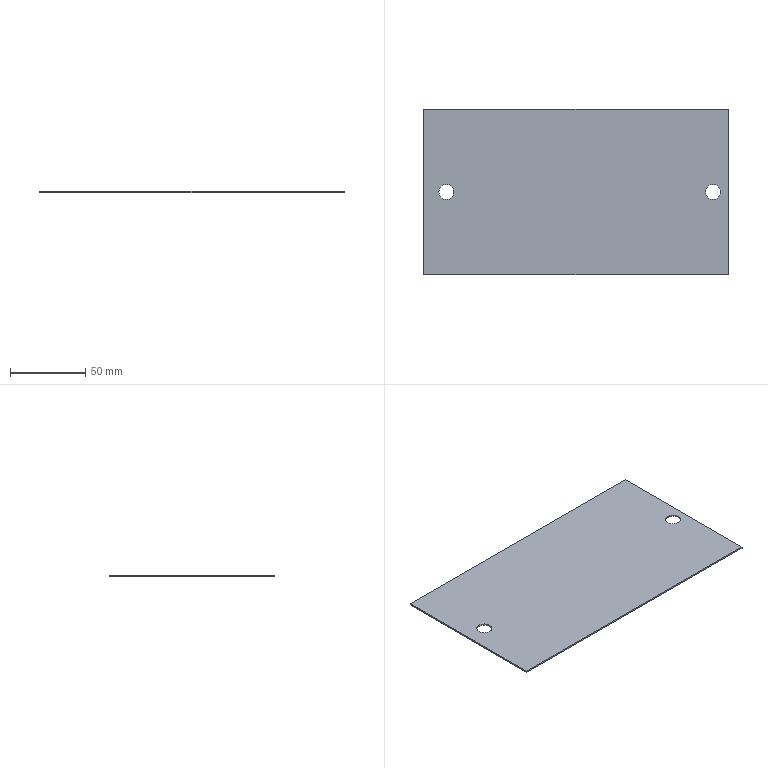Part | STEP file | 1 solid | 10 faces | box 202.5 x 110 x 1 mm | volume 22118 mm3 | plane 6 | cylinder 4 | commonest cylinder face diameters 10 x4
STEP:
#1=CARTESIAN_POINT('',(0.,0.,0.));
#2=DIRECTION('',(0.,0.,1.));
#3=DIRECTION('',(1.,0.,0.));
#4=AXIS2_PLACEMENT_3D('',#1,#2,#3);
#5=CARTESIAN_POINT('',(134.208,-8.441,1.));
#6=VERTEX_POINT('',#5);
#7=CARTESIAN_POINT('',(134.208,-8.441,0.));
#8=VERTEX_POINT('',#7);
#9=CARTESIAN_POINT('',(134.208,-8.441,1.));
#10=DIRECTION('',(0.,0.,-1.));
#11=VECTOR('',#10,1.);
#12=LINE('',#9,#11);
#13=CARTESIAN_POINT('',(139.208,-8.441,1.));
#14=DIRECTION('',(0.,0.,-1.));
#15=DIRECTION('',(-1.,0.,0.));
#16=AXIS2_PLACEMENT_3D('',#13,#14,#15);
#17=CYLINDRICAL_SURFACE('',#16,5.);
#18=CARTESIAN_POINT('',(6.283,0.));
#19=DIRECTION('',(0.,1.));
#20=VECTOR('',#19,1.);
#21=LINE('',#18,#20);
#22=(GEOMETRIC_REPRESENTATION_CONTEXT(2)PARAMETRIC_REPRESENTATION_CONTEXT()REPRESENTATION_CONTEXT('',''));
#23=DEFINITIONAL_REPRESENTATION('',(#21),#22);
#24=PCURVE('',#17,#23);
#25=CARTESIAN_POINT('',(139.208,-8.441,1.));
#26=DIRECTION('',(0.,0.,-1.));
#27=DIRECTION('',(-1.,0.,0.));
#28=AXIS2_PLACEMENT_3D('',#25,#26,#27);
#29=CYLINDRICAL_SURFACE('',#28,5.);
#30=CARTESIAN_POINT('',(0.,0.));
#31=DIRECTION('',(0.,1.));
#32=VECTOR('',#31,1.);
#33=LINE('',#30,#32);
#34=(GEOMETRIC_REPRESENTATION_CONTEXT(2)PARAMETRIC_REPRESENTATION_CONTEXT()REPRESENTATION_CONTEXT('',''));
#35=DEFINITIONAL_REPRESENTATION('',(#33),#34);
#36=PCURVE('',#29,#35);
#37=SURFACE_CURVE('',#12,(#24,#36),.PCURVE_S1.);
#38=EDGE_CURVE('',#6,#8,#37,.T.);
#39=ORIENTED_EDGE('',*,*,#38,.T.);
#40=CARTESIAN_POINT('',(144.208,-8.441,0.));
#41=VERTEX_POINT('',#40);
#42=CARTESIAN_POINT('',(139.208,-8.441,0.));
#43=DIRECTION('',(0.,0.,-1.));
#44=DIRECTION('',(-1.,0.,0.));
#45=AXIS2_PLACEMENT_3D('',#42,#43,#44);
#46=CIRCLE('',#45,5.);
#47=CARTESIAN_POINT('',(0.,1.));
#48=DIRECTION('',(1.,0.));
#49=VECTOR('',#48,1.);
#50=LINE('',#47,#49);
#51=(GEOMETRIC_REPRESENTATION_CONTEXT(2)PARAMETRIC_REPRESENTATION_CONTEXT()REPRESENTATION_CONTEXT('',''));
#52=DEFINITIONAL_REPRESENTATION('',(#50),#51);
#53=PCURVE('',#17,#52);
#54=CARTESIAN_POINT('',(47.958,-8.441,0.));
#55=DIRECTION('',(0.,0.,1.));
#56=DIRECTION('',(1.,0.,0.));
#57=AXIS2_PLACEMENT_3D('',#54,#55,#56);
#58=PLANE('',#57);
#59=CARTESIAN_POINT('',(86.25,0.));
#60=CARTESIAN_POINT('',(86.25,8.66));
#61=CARTESIAN_POINT('',(93.75,4.33));
#62=CARTESIAN_POINT('',(101.25,0.));
#63=CARTESIAN_POINT('',(93.75,-4.33));
#64=CARTESIAN_POINT('',(86.25,-8.66));
#65=CARTESIAN_POINT('',(86.25,0.));
#66=(BOUNDED_CURVE()B_SPLINE_CURVE(2,(#59,#60,#61,#62,#63,#64,#65),.UNSPECIFIED.,.T.,.F.)B_SPLINE_CURVE_WITH_KNOTS((1,2,2,2,2,1),(-2.094,0.,2.094,4.189,6.283,8.378),.UNSPECIFIED.)CURVE()GEOMETRIC_REPRESENTATION_ITEM()RATIONAL_B_SPLINE_CURVE((1.,0.5,1.,0.5,1.,0.5,1.))REPRESENTATION_ITEM(''));
#67=(GEOMETRIC_REPRESENTATION_CONTEXT(2)PARAMETRIC_REPRESENTATION_CONTEXT()REPRESENTATION_CONTEXT('',''));
#68=DEFINITIONAL_REPRESENTATION('',(#66),#67);
#69=PCURVE('',#58,#68);
#70=SURFACE_CURVE('',#46,(#53,#69),.PCURVE_S1.);
#71=EDGE_CURVE('',#41,#8,#70,.T.);
#72=ORIENTED_EDGE('',*,*,#71,.F.);
#73=CARTESIAN_POINT('',(144.208,-8.441,1.));
#74=VERTEX_POINT('',#73);
#75=CARTESIAN_POINT('',(144.208,-8.441,1.));
#76=DIRECTION('',(0.,0.,-1.));
#77=VECTOR('',#76,1.);
#78=LINE('',#75,#77);
#79=CARTESIAN_POINT('',(3.142,0.));
#80=DIRECTION('',(0.,1.));
#81=VECTOR('',#80,1.);
#82=LINE('',#79,#81);
#83=(GEOMETRIC_REPRESENTATION_CONTEXT(2)PARAMETRIC_REPRESENTATION_CONTEXT()REPRESENTATION_CONTEXT('',''));
#84=DEFINITIONAL_REPRESENTATION('',(#82),#83);
#85=PCURVE('',#17,#84);
#86=CARTESIAN_POINT('',(3.142,0.));
#87=DIRECTION('',(0.,1.));
#88=VECTOR('',#87,1.);
#89=LINE('',#86,#88);
#90=(GEOMETRIC_REPRESENTATION_CONTEXT(2)PARAMETRIC_REPRESENTATION_CONTEXT()REPRESENTATION_CONTEXT('',''));
#91=DEFINITIONAL_REPRESENTATION('',(#89),#90);
#92=PCURVE('',#29,#91);
#93=SURFACE_CURVE('',#78,(#85,#92),.PCURVE_S1.);
#94=EDGE_CURVE('',#74,#41,#93,.T.);
#95=ORIENTED_EDGE('',*,*,#94,.F.);
#96=CARTESIAN_POINT('',(139.208,-8.441,1.));
#97=DIRECTION('',(0.,0.,-1.));
#98=DIRECTION('',(-1.,0.,0.));
#99=AXIS2_PLACEMENT_3D('',#96,#97,#98);
#100=CIRCLE('',#99,5.);
#101=CARTESIAN_POINT('',(0.,0.));
#102=DIRECTION('',(1.,0.));
#103=VECTOR('',#102,1.);
#104=LINE('',#101,#103);
#105=(GEOMETRIC_REPRESENTATION_CONTEXT(2)PARAMETRIC_REPRESENTATION_CONTEXT()REPRESENTATION_CONTEXT('',''));
#106=DEFINITIONAL_REPRESENTATION('',(#104),#105);
#107=PCURVE('',#17,#106);
#108=CARTESIAN_POINT('',(47.958,-8.441,1.));
#109=DIRECTION('',(0.,0.,1.));
#110=DIRECTION('',(1.,0.,0.));
#111=AXIS2_PLACEMENT_3D('',#108,#109,#110);
#112=PLANE('',#111);
#113=CARTESIAN_POINT('',(86.25,0.));
#114=CARTESIAN_POINT('',(86.25,8.66));
#115=CARTESIAN_POINT('',(93.75,4.33));
#116=CARTESIAN_POINT('',(101.25,0.));
#117=CARTESIAN_POINT('',(93.75,-4.33));
#118=CARTESIAN_POINT('',(86.25,-8.66));
#119=CARTESIAN_POINT('',(86.25,0.));
#120=(BOUNDED_CURVE()B_SPLINE_CURVE(2,(#113,#114,#115,#116,#117,#118,#119),.UNSPECIFIED.,.T.,.F.)B_SPLINE_CURVE_WITH_KNOTS((1,2,2,2,2,1),(-2.094,0.,2.094,4.189,6.283,8.378),.UNSPECIFIED.)CURVE()GEOMETRIC_REPRESENTATION_ITEM()RATIONAL_B_SPLINE_CURVE((1.,0.5,1.,0.5,1.,0.5,1.))REPRESENTATION_ITEM(''));
#121=(GEOMETRIC_REPRESENTATION_CONTEXT(2)PARAMETRIC_REPRESENTATION_CONTEXT()REPRESENTATION_CONTEXT('',''));
#122=DEFINITIONAL_REPRESENTATION('',(#120),#121);
#123=PCURVE('',#112,#122);
#124=SURFACE_CURVE('',#100,(#107,#123),.PCURVE_S1.);
#125=EDGE_CURVE('',#74,#6,#124,.T.);
#126=ORIENTED_EDGE('',*,*,#125,.T.);
#127=EDGE_LOOP('',(#39,#72,#95,#126));
#128=FACE_BOUND('',#127,.F.);
#129=ADVANCED_FACE('',(#128),#17,.F.);
#130=CARTESIAN_POINT('',(-43.292,-8.441,1.));
#131=VERTEX_POINT('',#130);
#132=CARTESIAN_POINT('',(-43.292,-8.441,0.));
#133=VERTEX_POINT('',#132);
#134=CARTESIAN_POINT('',(-43.292,-8.441,1.));
#135=DIRECTION('',(0.,0.,-1.));
#136=VECTOR('',#135,1.);
#137=LINE('',#134,#136);
#138=CARTESIAN_POINT('',(-38.292,-8.441,1.));
#139=DIRECTION('',(0.,0.,-1.));
#140=DIRECTION('',(-1.,0.,0.));
#141=AXIS2_PLACEMENT_3D('',#138,#139,#140);
#142=CYLINDRICAL_SURFACE('',#141,5.);
#143=CARTESIAN_POINT('',(6.283,0.));
#144=DIRECTION('',(0.,1.));
#145=VECTOR('',#144,1.);
#146=LINE('',#143,#145);
#147=(GEOMETRIC_REPRESENTATION_CONTEXT(2)PARAMETRIC_REPRESENTATION_CONTEXT()REPRESENTATION_CONTEXT('',''));
#148=DEFINITIONAL_REPRESENTATION('',(#146),#147);
#149=PCURVE('',#142,#148);
#150=CARTESIAN_POINT('',(-38.292,-8.441,1.));
#151=DIRECTION('',(0.,0.,-1.));
#152=DIRECTION('',(-1.,0.,0.));
#153=AXIS2_PLACEMENT_3D('',#150,#151,#152);
#154=CYLINDRICAL_SURFACE('',#153,5.);
#155=CARTESIAN_POINT('',(0.,0.));
#156=DIRECTION('',(0.,1.));
#157=VECTOR('',#156,1.);
#158=LINE('',#155,#157);
#159=(GEOMETRIC_REPRESENTATION_CONTEXT(2)PARAMETRIC_REPRESENTATION_CONTEXT()REPRESENTATION_CONTEXT('',''));
#160=DEFINITIONAL_REPRESENTATION('',(#158),#159);
#161=PCURVE('',#154,#160);
#162=SURFACE_CURVE('',#137,(#149,#161),.PCURVE_S1.);
#163=EDGE_CURVE('',#131,#133,#162,.T.);
#164=ORIENTED_EDGE('',*,*,#163,.T.);
#165=CARTESIAN_POINT('',(-33.292,-8.441,0.));
#166=VERTEX_POINT('',#165);
#167=CARTESIAN_POINT('',(-38.292,-8.441,0.));
#168=DIRECTION('',(0.,0.,-1.));
#169=DIRECTION('',(-1.,0.,0.));
#170=AXIS2_PLACEMENT_3D('',#167,#168,#169);
#171=CIRCLE('',#170,5.);
#172=CARTESIAN_POINT('',(0.,1.));
#173=DIRECTION('',(1.,0.));
#174=VECTOR('',#173,1.);
#175=LINE('',#172,#174);
#176=(GEOMETRIC_REPRESENTATION_CONTEXT(2)PARAMETRIC_REPRESENTATION_CONTEXT()REPRESENTATION_CONTEXT('',''));
#177=DEFINITIONAL_REPRESENTATION('',(#175),#176);
#178=PCURVE('',#142,#177);
#179=CARTESIAN_POINT('',(-91.25,0.));
#180=CARTESIAN_POINT('',(-91.25,8.66));
#181=CARTESIAN_POINT('',(-83.75,4.33));
#182=CARTESIAN_POINT('',(-76.25,0.));
#183=CARTESIAN_POINT('',(-83.75,-4.33));
#184=CARTESIAN_POINT('',(-91.25,-8.66));
#185=CARTESIAN_POINT('',(-91.25,0.));
#186=(BOUNDED_CURVE()B_SPLINE_CURVE(2,(#179,#180,#181,#182,#183,#184,#185),.UNSPECIFIED.,.T.,.F.)B_SPLINE_CURVE_WITH_KNOTS((1,2,2,2,2,1),(-2.094,0.,2.094,4.189,6.283,8.378),.UNSPECIFIED.)CURVE()GEOMETRIC_REPRESENTATION_ITEM()RATIONAL_B_SPLINE_CURVE((1.,0.5,1.,0.5,1.,0.5,1.))REPRESENTATION_ITEM(''));
#187=(GEOMETRIC_REPRESENTATION_CONTEXT(2)PARAMETRIC_REPRESENTATION_CONTEXT()REPRESENTATION_CONTEXT('',''));
#188=DEFINITIONAL_REPRESENTATION('',(#186),#187);
#189=PCURVE('',#58,#188);
#190=SURFACE_CURVE('',#171,(#178,#189),.PCURVE_S1.);
#191=EDGE_CURVE('',#166,#133,#190,.T.);
#192=ORIENTED_EDGE('',*,*,#191,.F.);
#193=CARTESIAN_POINT('',(-33.292,-8.441,1.));
#194=VERTEX_POINT('',#193);
#195=CARTESIAN_POINT('',(-33.292,-8.441,1.));
#196=DIRECTION('',(0.,0.,-1.));
#197=VECTOR('',#196,1.);
#198=LINE('',#195,#197);
#199=CARTESIAN_POINT('',(3.142,0.));
#200=DIRECTION('',(0.,1.));
#201=VECTOR('',#200,1.);
#202=LINE('',#199,#201);
#203=(GEOMETRIC_REPRESENTATION_CONTEXT(2)PARAMETRIC_REPRESENTATION_CONTEXT()REPRESENTATION_CONTEXT('',''));
#204=DEFINITIONAL_REPRESENTATION('',(#202),#203);
#205=PCURVE('',#142,#204);
#206=CARTESIAN_POINT('',(3.142,0.));
#207=DIRECTION('',(0.,1.));
#208=VECTOR('',#207,1.);
#209=LINE('',#206,#208);
#210=(GEOMETRIC_REPRESENTATION_CONTEXT(2)PARAMETRIC_REPRESENTATION_CONTEXT()REPRESENTATION_CONTEXT('',''));
#211=DEFINITIONAL_REPRESENTATION('',(#209),#210);
#212=PCURVE('',#154,#211);
#213=SURFACE_CURVE('',#198,(#205,#212),.PCURVE_S1.);
#214=EDGE_CURVE('',#194,#166,#213,.T.);
#215=ORIENTED_EDGE('',*,*,#214,.F.);
#216=CARTESIAN_POINT('',(-38.292,-8.441,1.));
#217=DIRECTION('',(0.,0.,-1.));
#218=DIRECTION('',(-1.,0.,0.));
#219=AXIS2_PLACEMENT_3D('',#216,#217,#218);
#220=CIRCLE('',#219,5.);
#221=CARTESIAN_POINT('',(0.,0.));
#222=DIRECTION('',(1.,0.));
#223=VECTOR('',#222,1.);
#224=LINE('',#221,#223);
#225=(GEOMETRIC_REPRESENTATION_CONTEXT(2)PARAMETRIC_REPRESENTATION_CONTEXT()REPRESENTATION_CONTEXT('',''));
#226=DEFINITIONAL_REPRESENTATION('',(#224),#225);
#227=PCURVE('',#142,#226);
#228=CARTESIAN_POINT('',(-91.25,0.));
#229=CARTESIAN_POINT('',(-91.25,8.66));
#230=CARTESIAN_POINT('',(-83.75,4.33));
#231=CARTESIAN_POINT('',(-76.25,0.));
#232=CARTESIAN_POINT('',(-83.75,-4.33));
#233=CARTESIAN_POINT('',(-91.25,-8.66));
#234=CARTESIAN_POINT('',(-91.25,0.));
#235=(BOUNDED_CURVE()B_SPLINE_CURVE(2,(#228,#229,#230,#231,#232,#233,#234),.UNSPECIFIED.,.T.,.F.)B_SPLINE_CURVE_WITH_KNOTS((1,2,2,2,2,1),(-2.094,0.,2.094,4.189,6.283,8.378),.UNSPECIFIED.)CURVE()GEOMETRIC_REPRESENTATION_ITEM()RATIONAL_B_SPLINE_CURVE((1.,0.5,1.,0.5,1.,0.5,1.))REPRESENTATION_ITEM(''));
#236=(GEOMETRIC_REPRESENTATION_CONTEXT(2)PARAMETRIC_REPRESENTATION_CONTEXT()REPRESENTATION_CONTEXT('',''));
#237=DEFINITIONAL_REPRESENTATION('',(#235),#236);
#238=PCURVE('',#112,#237);
#239=SURFACE_CURVE('',#220,(#227,#238),.PCURVE_S1.);
#240=EDGE_CURVE('',#194,#131,#239,.T.);
#241=ORIENTED_EDGE('',*,*,#240,.T.);
#242=EDGE_LOOP('',(#164,#192,#215,#241));
#243=FACE_BOUND('',#242,.F.);
#244=ADVANCED_FACE('',(#243),#142,.F.);
#245=CARTESIAN_POINT('',(149.208,-63.441,0.));
#246=VERTEX_POINT('',#245);
#247=CARTESIAN_POINT('',(149.208,46.559,0.));
#248=VERTEX_POINT('',#247);
#249=CARTESIAN_POINT('',(149.208,-8.441,0.));
#250=DIRECTION('',(0.,1.,0.));
#251=VECTOR('',#250,1.);
#252=LINE('',#249,#251);
#253=CARTESIAN_POINT('',(101.25,0.));
#254=DIRECTION('',(0.,1.));
#255=VECTOR('',#254,1.);
#256=LINE('',#253,#255);
#257=(GEOMETRIC_REPRESENTATION_CONTEXT(2)PARAMETRIC_REPRESENTATION_CONTEXT()REPRESENTATION_CONTEXT('',''));
#258=DEFINITIONAL_REPRESENTATION('',(#256),#257);
#259=PCURVE('',#58,#258);
#260=CARTESIAN_POINT('',(149.208,-63.441,0.));
#261=DIRECTION('',(1.,0.,0.));
#262=DIRECTION('',(0.,0.,-1.));
#263=AXIS2_PLACEMENT_3D('',#260,#261,#262);
#264=PLANE('',#263);
#265=CARTESIAN_POINT('',(0.,55.));
#266=DIRECTION('',(0.,1.));
#267=VECTOR('',#266,1.);
#268=LINE('',#265,#267);
#269=(GEOMETRIC_REPRESENTATION_CONTEXT(2)PARAMETRIC_REPRESENTATION_CONTEXT()REPRESENTATION_CONTEXT('',''));
#270=DEFINITIONAL_REPRESENTATION('',(#268),#269);
#271=PCURVE('',#264,#270);
#272=SURFACE_CURVE('',#252,(#259,#271),.PCURVE_S1.);
#273=EDGE_CURVE('',#246,#248,#272,.T.);
#274=ORIENTED_EDGE('',*,*,#273,.F.);
#275=CARTESIAN_POINT('',(-53.292,-63.441,0.));
#276=VERTEX_POINT('',#275);
#277=CARTESIAN_POINT('',(47.958,-63.441,0.));
#278=DIRECTION('',(1.,0.,0.));
#279=VECTOR('',#278,1.);
#280=LINE('',#277,#279);
#281=CARTESIAN_POINT('',(0.,-55.));
#282=DIRECTION('',(1.,0.));
#283=VECTOR('',#282,1.);
#284=LINE('',#281,#283);
#285=(GEOMETRIC_REPRESENTATION_CONTEXT(2)PARAMETRIC_REPRESENTATION_CONTEXT()REPRESENTATION_CONTEXT('',''));
#286=DEFINITIONAL_REPRESENTATION('',(#284),#285);
#287=PCURVE('',#58,#286);
#288=CARTESIAN_POINT('',(-53.292,-63.441,0.));
#289=DIRECTION('',(0.,-1.,0.));
#290=DIRECTION('',(1.,0.,0.));
#291=AXIS2_PLACEMENT_3D('',#288,#289,#290);
#292=PLANE('',#291);
#293=CARTESIAN_POINT('',(101.25,0.));
#294=DIRECTION('',(1.,0.));
#295=VECTOR('',#294,1.);
#296=LINE('',#293,#295);
#297=(GEOMETRIC_REPRESENTATION_CONTEXT(2)PARAMETRIC_REPRESENTATION_CONTEXT()REPRESENTATION_CONTEXT('',''));
#298=DEFINITIONAL_REPRESENTATION('',(#296),#297);
#299=PCURVE('',#292,#298);
#300=SURFACE_CURVE('',#280,(#287,#299),.PCURVE_S1.);
#301=EDGE_CURVE('',#276,#246,#300,.T.);
#302=ORIENTED_EDGE('',*,*,#301,.F.);
#303=CARTESIAN_POINT('',(-53.292,46.559,0.));
#304=VERTEX_POINT('',#303);
#305=CARTESIAN_POINT('',(-53.292,-8.441,0.));
#306=DIRECTION('',(0.,-1.,0.));
#307=VECTOR('',#306,1.);
#308=LINE('',#305,#307);
#309=CARTESIAN_POINT('',(-101.25,0.));
#310=DIRECTION('',(0.,-1.));
#311=VECTOR('',#310,1.);
#312=LINE('',#309,#311);
#313=(GEOMETRIC_REPRESENTATION_CONTEXT(2)PARAMETRIC_REPRESENTATION_CONTEXT()REPRESENTATION_CONTEXT('',''));
#314=DEFINITIONAL_REPRESENTATION('',(#312),#313);
#315=PCURVE('',#58,#314);
#316=CARTESIAN_POINT('',(-53.292,46.559,0.));
#317=DIRECTION('',(-1.,0.,0.));
#318=DIRECTION('',(0.,-1.,0.));
#319=AXIS2_PLACEMENT_3D('',#316,#317,#318);
#320=PLANE('',#319);
#321=CARTESIAN_POINT('',(55.,0.));
#322=DIRECTION('',(1.,0.));
#323=VECTOR('',#322,1.);
#324=LINE('',#321,#323);
#325=(GEOMETRIC_REPRESENTATION_CONTEXT(2)PARAMETRIC_REPRESENTATION_CONTEXT()REPRESENTATION_CONTEXT('',''));
#326=DEFINITIONAL_REPRESENTATION('',(#324),#325);
#327=PCURVE('',#320,#326);
#328=SURFACE_CURVE('',#308,(#315,#327),.PCURVE_S1.);
#329=EDGE_CURVE('',#304,#276,#328,.T.);
#330=ORIENTED_EDGE('',*,*,#329,.F.);
#331=CARTESIAN_POINT('',(47.958,46.559,0.));
#332=DIRECTION('',(-1.,0.,0.));
#333=VECTOR('',#332,1.);
#334=LINE('',#331,#333);
#335=CARTESIAN_POINT('',(0.,55.));
#336=DIRECTION('',(-1.,0.));
#337=VECTOR('',#336,1.);
#338=LINE('',#335,#337);
#339=(GEOMETRIC_REPRESENTATION_CONTEXT(2)PARAMETRIC_REPRESENTATION_CONTEXT()REPRESENTATION_CONTEXT('',''));
#340=DEFINITIONAL_REPRESENTATION('',(#338),#339);
#341=PCURVE('',#58,#340);
#342=CARTESIAN_POINT('',(149.208,46.559,0.));
#343=DIRECTION('',(0.,1.,0.));
#344=DIRECTION('',(0.,0.,1.));
#345=AXIS2_PLACEMENT_3D('',#342,#343,#344);
#346=PLANE('',#345);
#347=CARTESIAN_POINT('',(0.,-101.25));
#348=DIRECTION('',(0.,-1.));
#349=VECTOR('',#348,1.);
#350=LINE('',#347,#349);
#351=(GEOMETRIC_REPRESENTATION_CONTEXT(2)PARAMETRIC_REPRESENTATION_CONTEXT()REPRESENTATION_CONTEXT('',''));
#352=DEFINITIONAL_REPRESENTATION('',(#350),#351);
#353=PCURVE('',#346,#352);
#354=SURFACE_CURVE('',#334,(#341,#353),.PCURVE_S1.);
#355=EDGE_CURVE('',#248,#304,#354,.T.);
#356=ORIENTED_EDGE('',*,*,#355,.F.);
#357=EDGE_LOOP('',(#274,#302,#330,#356));
#358=FACE_BOUND('',#357,.T.);
#359=CARTESIAN_POINT('',(139.208,-8.441,0.));
#360=DIRECTION('',(0.,0.,-1.));
#361=DIRECTION('',(-1.,0.,0.));
#362=AXIS2_PLACEMENT_3D('',#359,#360,#361);
#363=CIRCLE('',#362,5.);
#364=CARTESIAN_POINT('',(86.25,0.));
#365=CARTESIAN_POINT('',(86.25,8.66));
#366=CARTESIAN_POINT('',(93.75,4.33));
#367=CARTESIAN_POINT('',(101.25,0.));
#368=CARTESIAN_POINT('',(93.75,-4.33));
#369=CARTESIAN_POINT('',(86.25,-8.66));
#370=CARTESIAN_POINT('',(86.25,0.));
#371=(BOUNDED_CURVE()B_SPLINE_CURVE(2,(#364,#365,#366,#367,#368,#369,#370),.UNSPECIFIED.,.T.,.F.)B_SPLINE_CURVE_WITH_KNOTS((1,2,2,2,2,1),(-2.094,0.,2.094,4.189,6.283,8.378),.UNSPECIFIED.)CURVE()GEOMETRIC_REPRESENTATION_ITEM()RATIONAL_B_SPLINE_CURVE((1.,0.5,1.,0.5,1.,0.5,1.))REPRESENTATION_ITEM(''));
#372=(GEOMETRIC_REPRESENTATION_CONTEXT(2)PARAMETRIC_REPRESENTATION_CONTEXT()REPRESENTATION_CONTEXT('',''));
#373=DEFINITIONAL_REPRESENTATION('',(#371),#372);
#374=PCURVE('',#58,#373);
#375=CARTESIAN_POINT('',(0.,1.));
#376=DIRECTION('',(1.,0.));
#377=VECTOR('',#376,1.);
#378=LINE('',#375,#377);
#379=(GEOMETRIC_REPRESENTATION_CONTEXT(2)PARAMETRIC_REPRESENTATION_CONTEXT()REPRESENTATION_CONTEXT('',''));
#380=DEFINITIONAL_REPRESENTATION('',(#378),#379);
#381=PCURVE('',#29,#380);
#382=SURFACE_CURVE('',#363,(#374,#381),.PCURVE_S1.);
#383=EDGE_CURVE('',#8,#41,#382,.T.);
#384=ORIENTED_EDGE('',*,*,#383,.F.);
#385=ORIENTED_EDGE('',*,*,#71,.F.);
#386=EDGE_LOOP('',(#384,#385));
#387=FACE_BOUND('',#386,.T.);
#388=CARTESIAN_POINT('',(-38.292,-8.441,0.));
#389=DIRECTION('',(0.,0.,-1.));
#390=DIRECTION('',(-1.,0.,0.));
#391=AXIS2_PLACEMENT_3D('',#388,#389,#390);
#392=CIRCLE('',#391,5.);
#393=CARTESIAN_POINT('',(-91.25,0.));
#394=CARTESIAN_POINT('',(-91.25,8.66));
#395=CARTESIAN_POINT('',(-83.75,4.33));
#396=CARTESIAN_POINT('',(-76.25,0.));
#397=CARTESIAN_POINT('',(-83.75,-4.33));
#398=CARTESIAN_POINT('',(-91.25,-8.66));
#399=CARTESIAN_POINT('',(-91.25,0.));
#400=(BOUNDED_CURVE()B_SPLINE_CURVE(2,(#393,#394,#395,#396,#397,#398,#399),.UNSPECIFIED.,.T.,.F.)B_SPLINE_CURVE_WITH_KNOTS((1,2,2,2,2,1),(-2.094,0.,2.094,4.189,6.283,8.378),.UNSPECIFIED.)CURVE()GEOMETRIC_REPRESENTATION_ITEM()RATIONAL_B_SPLINE_CURVE((1.,0.5,1.,0.5,1.,0.5,1.))REPRESENTATION_ITEM(''));
#401=(GEOMETRIC_REPRESENTATION_CONTEXT(2)PARAMETRIC_REPRESENTATION_CONTEXT()REPRESENTATION_CONTEXT('',''));
#402=DEFINITIONAL_REPRESENTATION('',(#400),#401);
#403=PCURVE('',#58,#402);
#404=CARTESIAN_POINT('',(0.,1.));
#405=DIRECTION('',(1.,0.));
#406=VECTOR('',#405,1.);
#407=LINE('',#404,#406);
#408=(GEOMETRIC_REPRESENTATION_CONTEXT(2)PARAMETRIC_REPRESENTATION_CONTEXT()REPRESENTATION_CONTEXT('',''));
#409=DEFINITIONAL_REPRESENTATION('',(#407),#408);
#410=PCURVE('',#154,#409);
#411=SURFACE_CURVE('',#392,(#403,#410),.PCURVE_S1.);
#412=EDGE_CURVE('',#133,#166,#411,.T.);
#413=ORIENTED_EDGE('',*,*,#412,.F.);
#414=ORIENTED_EDGE('',*,*,#191,.F.);
#415=EDGE_LOOP('',(#413,#414));
#416=FACE_BOUND('',#415,.T.);
#417=ADVANCED_FACE('',(#358,#387,#416),#58,.F.);
#418=CARTESIAN_POINT('',(-53.292,46.559,1.));
#419=VERTEX_POINT('',#418);
#420=CARTESIAN_POINT('',(149.208,46.559,1.));
#421=VERTEX_POINT('',#420);
#422=CARTESIAN_POINT('',(149.208,46.559,1.));
#423=DIRECTION('',(1.,0.,0.));
#424=VECTOR('',#423,1.);
#425=LINE('',#422,#424);
#426=CARTESIAN_POINT('',(1.,0.));
#427=DIRECTION('',(0.,1.));
#428=VECTOR('',#427,1.);
#429=LINE('',#426,#428);
#430=(GEOMETRIC_REPRESENTATION_CONTEXT(2)PARAMETRIC_REPRESENTATION_CONTEXT()REPRESENTATION_CONTEXT('',''));
#431=DEFINITIONAL_REPRESENTATION('',(#429),#430);
#432=PCURVE('',#346,#431);
#433=CARTESIAN_POINT('',(101.25,55.));
#434=DIRECTION('',(1.,0.));
#435=VECTOR('',#434,1.);
#436=LINE('',#433,#435);
#437=(GEOMETRIC_REPRESENTATION_CONTEXT(2)PARAMETRIC_REPRESENTATION_CONTEXT()REPRESENTATION_CONTEXT('',''));
#438=DEFINITIONAL_REPRESENTATION('',(#436),#437);
#439=PCURVE('',#112,#438);
#440=SURFACE_CURVE('',#425,(#432,#439),.PCURVE_S1.);
#441=EDGE_CURVE('',#419,#421,#440,.T.);
#442=ORIENTED_EDGE('',*,*,#441,.T.);
#443=CARTESIAN_POINT('',(149.208,46.559,0.));
#444=DIRECTION('',(0.,0.,-1.));
#445=VECTOR('',#444,1.);
#446=LINE('',#443,#445);
#447=CARTESIAN_POINT('',(0.,0.));
#448=DIRECTION('',(-1.,0.));
#449=VECTOR('',#448,1.);
#450=LINE('',#447,#449);
#451=(GEOMETRIC_REPRESENTATION_CONTEXT(2)PARAMETRIC_REPRESENTATION_CONTEXT()REPRESENTATION_CONTEXT('',''));
#452=DEFINITIONAL_REPRESENTATION('',(#450),#451);
#453=PCURVE('',#346,#452);
#454=CARTESIAN_POINT('',(0.,110.));
#455=DIRECTION('',(1.,0.));
#456=VECTOR('',#455,1.);
#457=LINE('',#454,#456);
#458=(GEOMETRIC_REPRESENTATION_CONTEXT(2)PARAMETRIC_REPRESENTATION_CONTEXT()REPRESENTATION_CONTEXT('',''));
#459=DEFINITIONAL_REPRESENTATION('',(#457),#458);
#460=PCURVE('',#264,#459);
#461=SURFACE_CURVE('',#446,(#453,#460),.PCURVE_S1.);
#462=EDGE_CURVE('',#421,#248,#461,.T.);
#463=ORIENTED_EDGE('',*,*,#462,.T.);
#464=ORIENTED_EDGE('',*,*,#355,.T.);
#465=CARTESIAN_POINT('',(-53.292,46.559,0.));
#466=DIRECTION('',(0.,0.,1.));
#467=VECTOR('',#466,1.);
#468=LINE('',#465,#467);
#469=CARTESIAN_POINT('',(0.,-202.5));
#470=DIRECTION('',(1.,0.));
#471=VECTOR('',#470,1.);
#472=LINE('',#469,#471);
#473=(GEOMETRIC_REPRESENTATION_CONTEXT(2)PARAMETRIC_REPRESENTATION_CONTEXT()REPRESENTATION_CONTEXT('',''));
#474=DEFINITIONAL_REPRESENTATION('',(#472),#473);
#475=PCURVE('',#346,#474);
#476=CARTESIAN_POINT('',(0.,0.));
#477=DIRECTION('',(0.,1.));
#478=VECTOR('',#477,1.);
#479=LINE('',#476,#478);
#480=(GEOMETRIC_REPRESENTATION_CONTEXT(2)PARAMETRIC_REPRESENTATION_CONTEXT()REPRESENTATION_CONTEXT('',''));
#481=DEFINITIONAL_REPRESENTATION('',(#479),#480);
#482=PCURVE('',#320,#481);
#483=SURFACE_CURVE('',#468,(#475,#482),.PCURVE_S1.);
#484=EDGE_CURVE('',#304,#419,#483,.T.);
#485=ORIENTED_EDGE('',*,*,#484,.T.);
#486=EDGE_LOOP('',(#442,#463,#464,#485));
#487=FACE_BOUND('',#486,.T.);
#488=ADVANCED_FACE('',(#487),#346,.T.);
#489=CARTESIAN_POINT('',(149.208,-63.441,1.));
#490=VERTEX_POINT('',#489);
#491=CARTESIAN_POINT('',(149.208,-63.441,1.));
#492=DIRECTION('',(0.,-1.,0.));
#493=VECTOR('',#492,1.);
#494=LINE('',#491,#493);
#495=CARTESIAN_POINT('',(-1.,0.));
#496=DIRECTION('',(0.,-1.));
#497=VECTOR('',#496,1.);
#498=LINE('',#495,#497);
#499=(GEOMETRIC_REPRESENTATION_CONTEXT(2)PARAMETRIC_REPRESENTATION_CONTEXT()REPRESENTATION_CONTEXT('',''));
#500=DEFINITIONAL_REPRESENTATION('',(#498),#499);
#501=PCURVE('',#264,#500);
#502=CARTESIAN_POINT('',(101.25,-55.));
#503=DIRECTION('',(0.,-1.));
#504=VECTOR('',#503,1.);
#505=LINE('',#502,#504);
#506=(GEOMETRIC_REPRESENTATION_CONTEXT(2)PARAMETRIC_REPRESENTATION_CONTEXT()REPRESENTATION_CONTEXT('',''));
#507=DEFINITIONAL_REPRESENTATION('',(#505),#506);
#508=PCURVE('',#112,#507);
#509=SURFACE_CURVE('',#494,(#501,#508),.PCURVE_S1.);
#510=EDGE_CURVE('',#421,#490,#509,.T.);
#511=ORIENTED_EDGE('',*,*,#510,.T.);
#512=CARTESIAN_POINT('',(149.208,-63.441,0.));
#513=DIRECTION('',(0.,0.,-1.));
#514=VECTOR('',#513,1.);
#515=LINE('',#512,#514);
#516=CARTESIAN_POINT('',(0.,0.));
#517=DIRECTION('',(1.,0.));
#518=VECTOR('',#517,1.);
#519=LINE('',#516,#518);
#520=(GEOMETRIC_REPRESENTATION_CONTEXT(2)PARAMETRIC_REPRESENTATION_CONTEXT()REPRESENTATION_CONTEXT('',''));
#521=DEFINITIONAL_REPRESENTATION('',(#519),#520);
#522=PCURVE('',#264,#521);
#523=CARTESIAN_POINT('',(202.5,0.));
#524=DIRECTION('',(0.,-1.));
#525=VECTOR('',#524,1.);
#526=LINE('',#523,#525);
#527=(GEOMETRIC_REPRESENTATION_CONTEXT(2)PARAMETRIC_REPRESENTATION_CONTEXT()REPRESENTATION_CONTEXT('',''));
#528=DEFINITIONAL_REPRESENTATION('',(#526),#527);
#529=PCURVE('',#292,#528);
#530=SURFACE_CURVE('',#515,(#522,#529),.PCURVE_S1.);
#531=EDGE_CURVE('',#490,#246,#530,.T.);
#532=ORIENTED_EDGE('',*,*,#531,.T.);
#533=ORIENTED_EDGE('',*,*,#273,.T.);
#534=ORIENTED_EDGE('',*,*,#462,.F.);
#535=EDGE_LOOP('',(#511,#532,#533,#534));
#536=FACE_BOUND('',#535,.T.);
#537=ADVANCED_FACE('',(#536),#264,.T.);
#538=CARTESIAN_POINT('',(-53.292,-63.441,1.));
#539=VERTEX_POINT('',#538);
#540=CARTESIAN_POINT('',(-53.292,-63.441,1.));
#541=DIRECTION('',(-1.,0.,0.));
#542=VECTOR('',#541,1.);
#543=LINE('',#540,#542);
#544=CARTESIAN_POINT('',(0.,1.));
#545=DIRECTION('',(-1.,0.));
#546=VECTOR('',#545,1.);
#547=LINE('',#544,#546);
#548=(GEOMETRIC_REPRESENTATION_CONTEXT(2)PARAMETRIC_REPRESENTATION_CONTEXT()REPRESENTATION_CONTEXT('',''));
#549=DEFINITIONAL_REPRESENTATION('',(#547),#548);
#550=PCURVE('',#292,#549);
#551=CARTESIAN_POINT('',(-101.25,-55.));
#552=DIRECTION('',(-1.,0.));
#553=VECTOR('',#552,1.);
#554=LINE('',#551,#553);
#555=(GEOMETRIC_REPRESENTATION_CONTEXT(2)PARAMETRIC_REPRESENTATION_CONTEXT()REPRESENTATION_CONTEXT('',''));
#556=DEFINITIONAL_REPRESENTATION('',(#554),#555);
#557=PCURVE('',#112,#556);
#558=SURFACE_CURVE('',#543,(#550,#557),.PCURVE_S1.);
#559=EDGE_CURVE('',#490,#539,#558,.T.);
#560=ORIENTED_EDGE('',*,*,#559,.T.);
#561=CARTESIAN_POINT('',(-53.292,-63.441,0.));
#562=DIRECTION('',(0.,0.,-1.));
#563=VECTOR('',#562,1.);
#564=LINE('',#561,#563);
#565=CARTESIAN_POINT('',(0.,0.));
#566=DIRECTION('',(0.,-1.));
#567=VECTOR('',#566,1.);
#568=LINE('',#565,#567);
#569=(GEOMETRIC_REPRESENTATION_CONTEXT(2)PARAMETRIC_REPRESENTATION_CONTEXT()REPRESENTATION_CONTEXT('',''));
#570=DEFINITIONAL_REPRESENTATION('',(#568),#569);
#571=PCURVE('',#292,#570);
#572=CARTESIAN_POINT('',(110.,0.));
#573=DIRECTION('',(0.,-1.));
#574=VECTOR('',#573,1.);
#575=LINE('',#572,#574);
#576=(GEOMETRIC_REPRESENTATION_CONTEXT(2)PARAMETRIC_REPRESENTATION_CONTEXT()REPRESENTATION_CONTEXT('',''));
#577=DEFINITIONAL_REPRESENTATION('',(#575),#576);
#578=PCURVE('',#320,#577);
#579=SURFACE_CURVE('',#564,(#571,#578),.PCURVE_S1.);
#580=EDGE_CURVE('',#539,#276,#579,.T.);
#581=ORIENTED_EDGE('',*,*,#580,.T.);
#582=ORIENTED_EDGE('',*,*,#301,.T.);
#583=ORIENTED_EDGE('',*,*,#531,.F.);
#584=EDGE_LOOP('',(#560,#581,#582,#583));
#585=FACE_BOUND('',#584,.T.);
#586=ADVANCED_FACE('',(#585),#292,.T.);
#587=CARTESIAN_POINT('',(-53.292,46.559,1.));
#588=DIRECTION('',(0.,1.,0.));
#589=VECTOR('',#588,1.);
#590=LINE('',#587,#589);
#591=CARTESIAN_POINT('',(0.,1.));
#592=DIRECTION('',(-1.,0.));
#593=VECTOR('',#592,1.);
#594=LINE('',#591,#593);
#595=(GEOMETRIC_REPRESENTATION_CONTEXT(2)PARAMETRIC_REPRESENTATION_CONTEXT()REPRESENTATION_CONTEXT('',''));
#596=DEFINITIONAL_REPRESENTATION('',(#594),#595);
#597=PCURVE('',#320,#596);
#598=CARTESIAN_POINT('',(-101.25,55.));
#599=DIRECTION('',(0.,1.));
#600=VECTOR('',#599,1.);
#601=LINE('',#598,#600);
#602=(GEOMETRIC_REPRESENTATION_CONTEXT(2)PARAMETRIC_REPRESENTATION_CONTEXT()REPRESENTATION_CONTEXT('',''));
#603=DEFINITIONAL_REPRESENTATION('',(#601),#602);
#604=PCURVE('',#112,#603);
#605=SURFACE_CURVE('',#590,(#597,#604),.PCURVE_S1.);
#606=EDGE_CURVE('',#539,#419,#605,.T.);
#607=ORIENTED_EDGE('',*,*,#606,.T.);
#608=ORIENTED_EDGE('',*,*,#484,.F.);
#609=ORIENTED_EDGE('',*,*,#329,.T.);
#610=ORIENTED_EDGE('',*,*,#580,.F.);
#611=EDGE_LOOP('',(#607,#608,#609,#610));
#612=FACE_BOUND('',#611,.T.);
#613=ADVANCED_FACE('',(#612),#320,.T.);
#614=ORIENTED_EDGE('',*,*,#383,.F.);
#615=ORIENTED_EDGE('',*,*,#38,.F.);
#616=CARTESIAN_POINT('',(139.208,-8.441,1.));
#617=DIRECTION('',(0.,0.,-1.));
#618=DIRECTION('',(-1.,0.,0.));
#619=AXIS2_PLACEMENT_3D('',#616,#617,#618);
#620=CIRCLE('',#619,5.);
#621=CARTESIAN_POINT('',(0.,0.));
#622=DIRECTION('',(1.,0.));
#623=VECTOR('',#622,1.);
#624=LINE('',#621,#623);
#625=(GEOMETRIC_REPRESENTATION_CONTEXT(2)PARAMETRIC_REPRESENTATION_CONTEXT()REPRESENTATION_CONTEXT('',''));
#626=DEFINITIONAL_REPRESENTATION('',(#624),#625);
#627=PCURVE('',#29,#626);
#628=CARTESIAN_POINT('',(86.25,0.));
#629=CARTESIAN_POINT('',(86.25,8.66));
#630=CARTESIAN_POINT('',(93.75,4.33));
#631=CARTESIAN_POINT('',(101.25,0.));
#632=CARTESIAN_POINT('',(93.75,-4.33));
#633=CARTESIAN_POINT('',(86.25,-8.66));
#634=CARTESIAN_POINT('',(86.25,0.));
#635=(BOUNDED_CURVE()B_SPLINE_CURVE(2,(#628,#629,#630,#631,#632,#633,#634),.UNSPECIFIED.,.T.,.F.)B_SPLINE_CURVE_WITH_KNOTS((1,2,2,2,2,1),(-2.094,0.,2.094,4.189,6.283,8.378),.UNSPECIFIED.)CURVE()GEOMETRIC_REPRESENTATION_ITEM()RATIONAL_B_SPLINE_CURVE((1.,0.5,1.,0.5,1.,0.5,1.))REPRESENTATION_ITEM(''));
#636=(GEOMETRIC_REPRESENTATION_CONTEXT(2)PARAMETRIC_REPRESENTATION_CONTEXT()REPRESENTATION_CONTEXT('',''));
#637=DEFINITIONAL_REPRESENTATION('',(#635),#636);
#638=PCURVE('',#112,#637);
#639=SURFACE_CURVE('',#620,(#627,#638),.PCURVE_S1.);
#640=EDGE_CURVE('',#6,#74,#639,.T.);
#641=ORIENTED_EDGE('',*,*,#640,.T.);
#642=ORIENTED_EDGE('',*,*,#94,.T.);
#643=EDGE_LOOP('',(#614,#615,#641,#642));
#644=FACE_BOUND('',#643,.F.);
#645=ADVANCED_FACE('',(#644),#29,.F.);
#646=ORIENTED_EDGE('',*,*,#412,.F.);
#647=ORIENTED_EDGE('',*,*,#163,.F.);
#648=CARTESIAN_POINT('',(-38.292,-8.441,1.));
#649=DIRECTION('',(0.,0.,-1.));
#650=DIRECTION('',(-1.,0.,0.));
#651=AXIS2_PLACEMENT_3D('',#648,#649,#650);
#652=CIRCLE('',#651,5.);
#653=CARTESIAN_POINT('',(0.,0.));
#654=DIRECTION('',(1.,0.));
#655=VECTOR('',#654,1.);
#656=LINE('',#653,#655);
#657=(GEOMETRIC_REPRESENTATION_CONTEXT(2)PARAMETRIC_REPRESENTATION_CONTEXT()REPRESENTATION_CONTEXT('',''));
#658=DEFINITIONAL_REPRESENTATION('',(#656),#657);
#659=PCURVE('',#154,#658);
#660=CARTESIAN_POINT('',(-91.25,0.));
#661=CARTESIAN_POINT('',(-91.25,8.66));
#662=CARTESIAN_POINT('',(-83.75,4.33));
#663=CARTESIAN_POINT('',(-76.25,0.));
#664=CARTESIAN_POINT('',(-83.75,-4.33));
#665=CARTESIAN_POINT('',(-91.25,-8.66));
#666=CARTESIAN_POINT('',(-91.25,0.));
#667=(BOUNDED_CURVE()B_SPLINE_CURVE(2,(#660,#661,#662,#663,#664,#665,#666),.UNSPECIFIED.,.T.,.F.)B_SPLINE_CURVE_WITH_KNOTS((1,2,2,2,2,1),(-2.094,0.,2.094,4.189,6.283,8.378),.UNSPECIFIED.)CURVE()GEOMETRIC_REPRESENTATION_ITEM()RATIONAL_B_SPLINE_CURVE((1.,0.5,1.,0.5,1.,0.5,1.))REPRESENTATION_ITEM(''));
#668=(GEOMETRIC_REPRESENTATION_CONTEXT(2)PARAMETRIC_REPRESENTATION_CONTEXT()REPRESENTATION_CONTEXT('',''));
#669=DEFINITIONAL_REPRESENTATION('',(#667),#668);
#670=PCURVE('',#112,#669);
#671=SURFACE_CURVE('',#652,(#659,#670),.PCURVE_S1.);
#672=EDGE_CURVE('',#131,#194,#671,.T.);
#673=ORIENTED_EDGE('',*,*,#672,.T.);
#674=ORIENTED_EDGE('',*,*,#214,.T.);
#675=EDGE_LOOP('',(#646,#647,#673,#674));
#676=FACE_BOUND('',#675,.F.);
#677=ADVANCED_FACE('',(#676),#154,.F.);
#678=ORIENTED_EDGE('',*,*,#559,.F.);
#679=ORIENTED_EDGE('',*,*,#510,.F.);
#680=ORIENTED_EDGE('',*,*,#441,.F.);
#681=ORIENTED_EDGE('',*,*,#606,.F.);
#682=EDGE_LOOP('',(#678,#679,#680,#681));
#683=FACE_BOUND('',#682,.T.);
#684=ORIENTED_EDGE('',*,*,#640,.T.);
#685=ORIENTED_EDGE('',*,*,#125,.T.);
#686=EDGE_LOOP('',(#684,#685));
#687=FACE_BOUND('',#686,.T.);
#688=ORIENTED_EDGE('',*,*,#672,.T.);
#689=ORIENTED_EDGE('',*,*,#240,.T.);
#690=EDGE_LOOP('',(#688,#689));
#691=FACE_BOUND('',#690,.T.);
#692=ADVANCED_FACE('',(#683,#687,#691),#112,.T.);
#693=CLOSED_SHELL('',(#129,#244,#417,#488,#537,#586,#613,#645,#677,#692));
#694=MANIFOLD_SOLID_BREP('',#693);
#695=(LENGTH_UNIT()NAMED_UNIT(*)SI_UNIT(.MILLI.,.METRE.));
#696=UNCERTAINTY_MEASURE_WITH_UNIT(LENGTH_MEASURE(0.0000001),#695,'','');
#697=(NAMED_UNIT(*)PLANE_ANGLE_UNIT()SI_UNIT($,.RADIAN.));
#698=(NAMED_UNIT(*)SI_UNIT($,.STERADIAN.)SOLID_ANGLE_UNIT());
#699=(GEOMETRIC_REPRESENTATION_CONTEXT(3)GLOBAL_UNCERTAINTY_ASSIGNED_CONTEXT((#696))GLOBAL_UNIT_ASSIGNED_CONTEXT((#695,#697,#698))REPRESENTATION_CONTEXT('',''));
#700=ADVANCED_BREP_SHAPE_REPRESENTATION('',(#4,#694),#699);